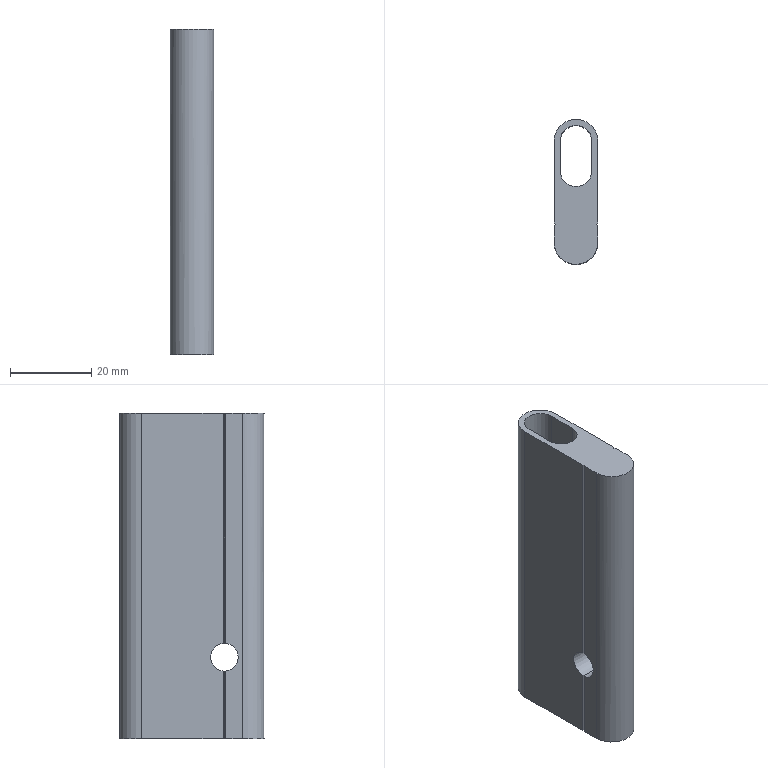Part | STEP file | 46A-01005CC13 | 1 solid | 22 faces | box 10.8 x 35.7 x 80 mm | volume 20059 mm3 | plane 16 | cylinder 6 | commonest cylinder face diameters 6.8 x2 7.8 x2 10.8 x2
STEP:
#1=CARTESIAN_POINT('',(-5.1,-8.,23.4));
#2=VERTEX_POINT('',#1);
#3=CARTESIAN_POINT('',(-5.4,-8.3,23.387));
#4=VERTEX_POINT('',#3);
#5=CARTESIAN_POINT('',(-5.1,-8.,23.4));
#6=CARTESIAN_POINT('',(-5.2,-8.1,23.4));
#7=CARTESIAN_POINT('',(-5.3,-8.2,23.396));
#8=CARTESIAN_POINT('',(-5.4,-8.3,23.387));
#9=B_SPLINE_CURVE_WITH_KNOTS('',3,(#5,#6,#7,#8),.UNSPECIFIED.,.F.,.U.,(4,4),(0.,0.6004),.UNSPECIFIED.);
#10=EDGE_CURVE('',#2,#4,#9,.T.);
#11=ORIENTED_EDGE('',*,*,#10,.F.);
#12=CARTESIAN_POINT('',(5.1,-8.,23.4));
#13=VERTEX_POINT('',#12);
#14=CARTESIAN_POINT('',(5.4,-8.,23.4));
#15=DIRECTION('',(1.,0.,0.));
#16=VECTOR('',#15,1.);
#17=LINE('',#14,#16);
#18=EDGE_CURVE('',#2,#13,#17,.T.);
#19=ORIENTED_EDGE('',*,*,#18,.T.);
#20=CARTESIAN_POINT('',(5.4,-8.3,23.387));
#21=VERTEX_POINT('',#20);
#22=CARTESIAN_POINT('',(5.4,-8.3,23.387));
#23=CARTESIAN_POINT('',(5.3,-8.2,23.396));
#24=CARTESIAN_POINT('',(5.2,-8.1,23.4));
#25=CARTESIAN_POINT('',(5.1,-8.,23.4));
#26=B_SPLINE_CURVE_WITH_KNOTS('',3,(#22,#23,#24,#25),.UNSPECIFIED.,.F.,.U.,(4,4),(0.,0.6004),.UNSPECIFIED.);
#27=EDGE_CURVE('',#21,#13,#26,.T.);
#28=ORIENTED_EDGE('',*,*,#27,.F.);
#29=CARTESIAN_POINT('',(5.4,-8.3,16.613));
#30=VERTEX_POINT('',#29);
#31=CARTESIAN_POINT('',(5.4,-8.,20.));
#32=DIRECTION('',(1.,0.,0.));
#33=AXIS2_PLACEMENT_3D('',#31,#32,$);
#34=CIRCLE('',#33,3.4);
#35=EDGE_CURVE('',#21,#30,#34,.T.);
#36=ORIENTED_EDGE('',*,*,#35,.T.);
#37=CARTESIAN_POINT('',(5.1,-8.,16.6));
#38=VERTEX_POINT('',#37);
#39=CARTESIAN_POINT('',(5.1,-8.,16.6));
#40=CARTESIAN_POINT('',(5.2,-8.1,16.6));
#41=CARTESIAN_POINT('',(5.3,-8.2,16.604));
#42=CARTESIAN_POINT('',(5.4,-8.3,16.613));
#43=B_SPLINE_CURVE_WITH_KNOTS('',3,(#39,#40,#41,#42),.UNSPECIFIED.,.F.,.U.,(4,4),(0.,0.6004),.UNSPECIFIED.);
#44=EDGE_CURVE('',#38,#30,#43,.T.);
#45=ORIENTED_EDGE('',*,*,#44,.F.);
#46=CARTESIAN_POINT('',(-5.1,-8.,16.6));
#47=VERTEX_POINT('',#46);
#48=CARTESIAN_POINT('',(5.4,-8.,16.6));
#49=DIRECTION('',(1.,0.,0.));
#50=VECTOR('',#49,1.);
#51=LINE('',#48,#50);
#52=EDGE_CURVE('',#47,#38,#51,.T.);
#53=ORIENTED_EDGE('',*,*,#52,.F.);
#54=CARTESIAN_POINT('',(-5.4,-8.3,16.613));
#55=VERTEX_POINT('',#54);
#56=CARTESIAN_POINT('',(-5.4,-8.3,16.613));
#57=CARTESIAN_POINT('',(-5.3,-8.2,16.604));
#58=CARTESIAN_POINT('',(-5.2,-8.1,16.6));
#59=CARTESIAN_POINT('',(-5.1,-8.,16.6));
#60=B_SPLINE_CURVE_WITH_KNOTS('',3,(#56,#57,#58,#59),.UNSPECIFIED.,.F.,.U.,(4,4),(0.,0.6004),.UNSPECIFIED.);
#61=EDGE_CURVE('',#55,#47,#60,.T.);
#62=ORIENTED_EDGE('',*,*,#61,.F.);
#63=CARTESIAN_POINT('',(-5.4,-8.,20.));
#64=DIRECTION('',(1.,0.,0.));
#65=AXIS2_PLACEMENT_3D('',#63,#64,$);
#66=CIRCLE('',#65,3.4);
#67=EDGE_CURVE('',#4,#55,#66,.T.);
#68=ORIENTED_EDGE('',*,*,#67,.F.);
#69=EDGE_LOOP('',(#11,#19,#28,#36,#45,#53,#62,#68));
#70=FACE_OUTER_BOUND('',#69,.T.);
#71=CARTESIAN_POINT('',(5.4,-8.,20.));
#72=DIRECTION('',(1.,0.,0.));
#73=DIRECTION('',(0.,0.,1.));
#74=AXIS2_PLACEMENT_3D('',#71,#72,#73);
#75=CYLINDRICAL_SURFACE('',#74,3.4);
#76=ADVANCED_FACE('',(#70),#75,.F.);
#77=CARTESIAN_POINT('',(-5.1,-8.,80.));
#78=VERTEX_POINT('',#77);
#79=CARTESIAN_POINT('',(-5.1,-8.,51.7));
#80=DIRECTION('',(0.,0.,1.));
#81=VECTOR('',#80,1.);
#82=LINE('',#79,#81);
#83=EDGE_CURVE('',#2,#78,#82,.T.);
#84=ORIENTED_EDGE('',*,*,#83,.F.);
#85=ORIENTED_EDGE('',*,*,#10,.T.);
#86=CARTESIAN_POINT('',(-5.4,-8.3,80.));
#87=VERTEX_POINT('',#86);
#88=CARTESIAN_POINT('',(-5.4,-8.3,51.693));
#89=DIRECTION('',(0.,0.,1.));
#90=VECTOR('',#89,1.);
#91=LINE('',#88,#90);
#92=EDGE_CURVE('',#4,#87,#91,.T.);
#93=ORIENTED_EDGE('',*,*,#92,.T.);
#94=CARTESIAN_POINT('',(-5.25,-8.15,80.));
#95=DIRECTION('',(0.7071,0.7071,0.));
#96=VECTOR('',#95,1.);
#97=LINE('',#94,#96);
#98=EDGE_CURVE('',#87,#78,#97,.T.);
#99=ORIENTED_EDGE('',*,*,#98,.T.);
#100=EDGE_LOOP('',(#84,#85,#93,#99));
#101=FACE_OUTER_BOUND('',#100,.T.);
#102=CARTESIAN_POINT('',(-5.4,-8.3,-20.));
#103=DIRECTION('',(0.7071,-0.7071,0.));
#104=DIRECTION('',(0.7071,0.7071,0.));
#105=AXIS2_PLACEMENT_3D('',#102,#103,#104);
#106=PLANE('',#105);
#107=ADVANCED_FACE('',(#101),#106,.F.);
#108=ORIENTED_EDGE('',*,*,#18,.F.);
#109=CARTESIAN_POINT('',(-5.4,-7.7,23.387));
#110=VERTEX_POINT('',#109);
#111=CARTESIAN_POINT('',(-5.4,-7.7,23.387));
#112=CARTESIAN_POINT('',(-5.3,-7.8,23.396));
#113=CARTESIAN_POINT('',(-5.2,-7.9,23.4));
#114=CARTESIAN_POINT('',(-5.1,-8.,23.4));
#115=B_SPLINE_CURVE_WITH_KNOTS('',3,(#111,#112,#113,#114),.UNSPECIFIED.,.F.,.U.,(4,4),(0.,0.6004),.UNSPECIFIED.);
#116=EDGE_CURVE('',#110,#2,#115,.T.);
#117=ORIENTED_EDGE('',*,*,#116,.F.);
#118=CARTESIAN_POINT('',(-5.4,-7.7,16.613));
#119=VERTEX_POINT('',#118);
#120=CARTESIAN_POINT('',(-5.4,-8.,20.));
#121=DIRECTION('',(1.,0.,0.));
#122=AXIS2_PLACEMENT_3D('',#120,#121,$);
#123=CIRCLE('',#122,3.4);
#124=EDGE_CURVE('',#119,#110,#123,.T.);
#125=ORIENTED_EDGE('',*,*,#124,.F.);
#126=CARTESIAN_POINT('',(-5.1,-8.,16.6));
#127=CARTESIAN_POINT('',(-5.2,-7.9,16.6));
#128=CARTESIAN_POINT('',(-5.3,-7.8,16.604));
#129=CARTESIAN_POINT('',(-5.4,-7.7,16.613));
#130=B_SPLINE_CURVE_WITH_KNOTS('',3,(#126,#127,#128,#129),.UNSPECIFIED.,.F.,.U.,(4,4),(0.,0.6004),.UNSPECIFIED.);
#131=EDGE_CURVE('',#47,#119,#130,.T.);
#132=ORIENTED_EDGE('',*,*,#131,.F.);
#133=ORIENTED_EDGE('',*,*,#52,.T.);
#134=CARTESIAN_POINT('',(5.4,-7.7,16.613));
#135=VERTEX_POINT('',#134);
#136=CARTESIAN_POINT('',(5.4,-7.7,16.613));
#137=CARTESIAN_POINT('',(5.3,-7.8,16.604));
#138=CARTESIAN_POINT('',(5.2,-7.9,16.6));
#139=CARTESIAN_POINT('',(5.1,-8.,16.6));
#140=B_SPLINE_CURVE_WITH_KNOTS('',3,(#136,#137,#138,#139),.UNSPECIFIED.,.F.,.U.,(4,4),(0.,0.6004),.UNSPECIFIED.);
#141=EDGE_CURVE('',#135,#38,#140,.T.);
#142=ORIENTED_EDGE('',*,*,#141,.F.);
#143=CARTESIAN_POINT('',(5.4,-7.7,23.387));
#144=VERTEX_POINT('',#143);
#145=CARTESIAN_POINT('',(5.4,-8.,20.));
#146=DIRECTION('',(1.,0.,0.));
#147=AXIS2_PLACEMENT_3D('',#145,#146,$);
#148=CIRCLE('',#147,3.4);
#149=EDGE_CURVE('',#135,#144,#148,.T.);
#150=ORIENTED_EDGE('',*,*,#149,.T.);
#151=CARTESIAN_POINT('',(5.1,-8.,23.4));
#152=CARTESIAN_POINT('',(5.2,-7.9,23.4));
#153=CARTESIAN_POINT('',(5.3,-7.8,23.396));
#154=CARTESIAN_POINT('',(5.4,-7.7,23.387));
#155=B_SPLINE_CURVE_WITH_KNOTS('',3,(#151,#152,#153,#154),.UNSPECIFIED.,.F.,.U.,(4,4),(0.,0.6004),.UNSPECIFIED.);
#156=EDGE_CURVE('',#13,#144,#155,.T.);
#157=ORIENTED_EDGE('',*,*,#156,.F.);
#158=EDGE_LOOP('',(#108,#117,#125,#132,#133,#142,#150,#157));
#159=FACE_OUTER_BOUND('',#158,.T.);
#160=CARTESIAN_POINT('',(5.4,-8.,20.));
#161=DIRECTION('',(1.,0.,0.));
#162=DIRECTION('',(0.,0.,-1.));
#163=AXIS2_PLACEMENT_3D('',#160,#161,#162);
#164=CYLINDRICAL_SURFACE('',#163,3.4);
#165=ADVANCED_FACE('',(#159),#164,.F.);
#166=CARTESIAN_POINT('',(5.4,-8.3,80.));
#167=VERTEX_POINT('',#166);
#168=CARTESIAN_POINT('',(5.4,-8.3,51.693));
#169=DIRECTION('',(0.,0.,1.));
#170=VECTOR('',#169,1.);
#171=LINE('',#168,#170);
#172=EDGE_CURVE('',#21,#167,#171,.T.);
#173=ORIENTED_EDGE('',*,*,#172,.F.);
#174=ORIENTED_EDGE('',*,*,#27,.T.);
#175=CARTESIAN_POINT('',(5.1,-8.,80.));
#176=VERTEX_POINT('',#175);
#177=CARTESIAN_POINT('',(5.1,-8.,51.7));
#178=DIRECTION('',(0.,0.,1.));
#179=VECTOR('',#178,1.);
#180=LINE('',#177,#179);
#181=EDGE_CURVE('',#13,#176,#180,.T.);
#182=ORIENTED_EDGE('',*,*,#181,.T.);
#183=CARTESIAN_POINT('',(5.25,-8.15,80.));
#184=DIRECTION('',(0.7071,-0.7071,0.));
#185=VECTOR('',#184,1.);
#186=LINE('',#183,#185);
#187=EDGE_CURVE('',#176,#167,#186,.T.);
#188=ORIENTED_EDGE('',*,*,#187,.T.);
#189=EDGE_LOOP('',(#173,#174,#182,#188));
#190=FACE_OUTER_BOUND('',#189,.T.);
#191=CARTESIAN_POINT('',(5.4,-8.3,-20.));
#192=DIRECTION('',(-0.7071,-0.7071,0.));
#193=DIRECTION('',(0.7071,-0.7071,0.));
#194=AXIS2_PLACEMENT_3D('',#191,#192,#193);
#195=PLANE('',#194);
#196=ADVANCED_FACE('',(#190),#195,.F.);
#197=CARTESIAN_POINT('',(5.4,-8.3,0.));
#198=VERTEX_POINT('',#197);
#199=CARTESIAN_POINT('',(5.4,-8.3,8.307));
#200=DIRECTION('',(0.,0.,1.));
#201=VECTOR('',#200,1.);
#202=LINE('',#199,#201);
#203=EDGE_CURVE('',#198,#30,#202,.T.);
#204=ORIENTED_EDGE('',*,*,#203,.T.);
#205=ORIENTED_EDGE('',*,*,#35,.F.);
#206=ORIENTED_EDGE('',*,*,#172,.T.);
#207=CARTESIAN_POINT('',(5.4,-12.45,80.));
#208=VERTEX_POINT('',#207);
#209=CARTESIAN_POINT('',(5.4,-10.375,80.));
#210=DIRECTION('',(0.,1.,0.));
#211=VECTOR('',#210,1.);
#212=LINE('',#209,#211);
#213=EDGE_CURVE('',#208,#167,#212,.T.);
#214=ORIENTED_EDGE('',*,*,#213,.F.);
#215=CARTESIAN_POINT('',(5.4,-12.45,0.));
#216=VERTEX_POINT('',#215);
#217=CARTESIAN_POINT('',(5.4,-12.45,40.));
#218=DIRECTION('',(0.,0.,-1.));
#219=VECTOR('',#218,1.);
#220=LINE('',#217,#219);
#221=EDGE_CURVE('',#208,#216,#220,.T.);
#222=ORIENTED_EDGE('',*,*,#221,.T.);
#223=CARTESIAN_POINT('',(5.4,-10.375,0.));
#224=DIRECTION('',(0.,1.,0.));
#225=VECTOR('',#224,1.);
#226=LINE('',#223,#225);
#227=EDGE_CURVE('',#216,#198,#226,.T.);
#228=ORIENTED_EDGE('',*,*,#227,.T.);
#229=EDGE_LOOP('',(#204,#205,#206,#214,#222,#228));
#230=FACE_OUTER_BOUND('',#229,.T.);
#231=CARTESIAN_POINT('',(5.4,-12.45,80.));
#232=DIRECTION('',(-1.,0.,0.));
#233=DIRECTION('',(0.,0.,1.));
#234=AXIS2_PLACEMENT_3D('',#231,#232,#233);
#235=PLANE('',#234);
#236=ADVANCED_FACE('',(#230),#235,.F.);
#237=CARTESIAN_POINT('',(5.1,-8.,0.));
#238=VERTEX_POINT('',#237);
#239=CARTESIAN_POINT('',(5.1,-8.,8.3));
#240=DIRECTION('',(0.,0.,1.));
#241=VECTOR('',#240,1.);
#242=LINE('',#239,#241);
#243=EDGE_CURVE('',#238,#38,#242,.T.);
#244=ORIENTED_EDGE('',*,*,#243,.T.);
#245=ORIENTED_EDGE('',*,*,#44,.T.);
#246=ORIENTED_EDGE('',*,*,#203,.F.);
#247=CARTESIAN_POINT('',(5.25,-8.15,0.));
#248=DIRECTION('',(0.7071,-0.7071,0.));
#249=VECTOR('',#248,1.);
#250=LINE('',#247,#249);
#251=EDGE_CURVE('',#238,#198,#250,.T.);
#252=ORIENTED_EDGE('',*,*,#251,.F.);
#253=EDGE_LOOP('',(#244,#245,#246,#252));
#254=FACE_OUTER_BOUND('',#253,.T.);
#255=CARTESIAN_POINT('',(5.4,-8.3,-20.));
#256=DIRECTION('',(-0.7071,-0.7071,0.));
#257=DIRECTION('',(0.7071,-0.7071,0.));
#258=AXIS2_PLACEMENT_3D('',#255,#256,#257);
#259=PLANE('',#258);
#260=ADVANCED_FACE('',(#254),#259,.F.);
#261=CARTESIAN_POINT('',(-5.4,-8.3,0.));
#262=VERTEX_POINT('',#261);
#263=CARTESIAN_POINT('',(-5.4,-8.3,8.307));
#264=DIRECTION('',(0.,0.,1.));
#265=VECTOR('',#264,1.);
#266=LINE('',#263,#265);
#267=EDGE_CURVE('',#262,#55,#266,.T.);
#268=ORIENTED_EDGE('',*,*,#267,.T.);
#269=ORIENTED_EDGE('',*,*,#61,.T.);
#270=CARTESIAN_POINT('',(-5.1,-8.,0.));
#271=VERTEX_POINT('',#270);
#272=CARTESIAN_POINT('',(-5.1,-8.,8.3));
#273=DIRECTION('',(0.,0.,1.));
#274=VECTOR('',#273,1.);
#275=LINE('',#272,#274);
#276=EDGE_CURVE('',#271,#47,#275,.T.);
#277=ORIENTED_EDGE('',*,*,#276,.F.);
#278=CARTESIAN_POINT('',(-5.25,-8.15,0.));
#279=DIRECTION('',(0.7071,0.7071,0.));
#280=VECTOR('',#279,1.);
#281=LINE('',#278,#280);
#282=EDGE_CURVE('',#262,#271,#281,.T.);
#283=ORIENTED_EDGE('',*,*,#282,.F.);
#284=EDGE_LOOP('',(#268,#269,#277,#283));
#285=FACE_OUTER_BOUND('',#284,.T.);
#286=CARTESIAN_POINT('',(-5.4,-8.3,-20.));
#287=DIRECTION('',(0.7071,-0.7071,0.));
#288=DIRECTION('',(0.7071,0.7071,0.));
#289=AXIS2_PLACEMENT_3D('',#286,#287,#288);
#290=PLANE('',#289);
#291=ADVANCED_FACE('',(#285),#290,.F.);
#292=ORIENTED_EDGE('',*,*,#67,.T.);
#293=ORIENTED_EDGE('',*,*,#267,.F.);
#294=CARTESIAN_POINT('',(-5.4,-12.45,0.));
#295=VERTEX_POINT('',#294);
#296=CARTESIAN_POINT('',(-5.4,-10.375,0.));
#297=DIRECTION('',(0.,1.,0.));
#298=VECTOR('',#297,1.);
#299=LINE('',#296,#298);
#300=EDGE_CURVE('',#295,#262,#299,.T.);
#301=ORIENTED_EDGE('',*,*,#300,.F.);
#302=CARTESIAN_POINT('',(-5.4,-12.45,80.));
#303=VERTEX_POINT('',#302);
#304=CARTESIAN_POINT('',(-5.4,-12.45,40.));
#305=DIRECTION('',(0.,0.,-1.));
#306=VECTOR('',#305,1.);
#307=LINE('',#304,#306);
#308=EDGE_CURVE('',#303,#295,#307,.T.);
#309=ORIENTED_EDGE('',*,*,#308,.F.);
#310=CARTESIAN_POINT('',(-5.4,-10.375,80.));
#311=DIRECTION('',(0.,1.,0.));
#312=VECTOR('',#311,1.);
#313=LINE('',#310,#312);
#314=EDGE_CURVE('',#303,#87,#313,.T.);
#315=ORIENTED_EDGE('',*,*,#314,.T.);
#316=ORIENTED_EDGE('',*,*,#92,.F.);
#317=EDGE_LOOP('',(#292,#293,#301,#309,#315,#316));
#318=FACE_OUTER_BOUND('',#317,.T.);
#319=CARTESIAN_POINT('',(-5.4,-12.45,80.));
#320=DIRECTION('',(-1.,0.,0.));
#321=DIRECTION('',(0.,-1.,0.));
#322=AXIS2_PLACEMENT_3D('',#319,#320,#321);
#323=PLANE('',#322);
#324=ADVANCED_FACE('',(#318),#323,.T.);
#325=CARTESIAN_POINT('',(-5.4,-7.7,80.));
#326=VERTEX_POINT('',#325);
#327=CARTESIAN_POINT('',(-5.4,-7.7,51.693));
#328=DIRECTION('',(0.,0.,1.));
#329=VECTOR('',#328,1.);
#330=LINE('',#327,#329);
#331=EDGE_CURVE('',#110,#326,#330,.T.);
#332=ORIENTED_EDGE('',*,*,#331,.F.);
#333=ORIENTED_EDGE('',*,*,#116,.T.);
#334=ORIENTED_EDGE('',*,*,#83,.T.);
#335=CARTESIAN_POINT('',(-5.25,-7.85,80.));
#336=DIRECTION('',(-0.7071,0.7071,0.));
#337=VECTOR('',#336,1.);
#338=LINE('',#335,#337);
#339=EDGE_CURVE('',#78,#326,#338,.T.);
#340=ORIENTED_EDGE('',*,*,#339,.T.);
#341=EDGE_LOOP('',(#332,#333,#334,#340));
#342=FACE_OUTER_BOUND('',#341,.T.);
#343=CARTESIAN_POINT('',(-5.4,-7.7,-20.));
#344=DIRECTION('',(0.7071,0.7071,0.));
#345=DIRECTION('',(-0.7071,0.7071,0.));
#346=AXIS2_PLACEMENT_3D('',#343,#344,#345);
#347=PLANE('',#346);
#348=ADVANCED_FACE('',(#342),#347,.F.);
#349=CARTESIAN_POINT('',(5.4,-7.7,80.));
#350=VERTEX_POINT('',#349);
#351=CARTESIAN_POINT('',(5.25,-7.85,80.));
#352=DIRECTION('',(-0.7071,-0.7071,0.));
#353=VECTOR('',#352,1.);
#354=LINE('',#351,#353);
#355=EDGE_CURVE('',#350,#176,#354,.T.);
#356=ORIENTED_EDGE('',*,*,#355,.F.);
#357=CARTESIAN_POINT('',(5.4,12.45,80.));
#358=VERTEX_POINT('',#357);
#359=CARTESIAN_POINT('',(5.4,2.375,80.));
#360=DIRECTION('',(0.,1.,0.));
#361=VECTOR('',#360,1.);
#362=LINE('',#359,#361);
#363=EDGE_CURVE('',#350,#358,#362,.T.);
#364=ORIENTED_EDGE('',*,*,#363,.T.);
#365=CARTESIAN_POINT('',(-5.4,12.45,80.));
#366=VERTEX_POINT('',#365);
#367=CARTESIAN_POINT('',(0.,12.45,80.));
#368=DIRECTION('',(0.,0.,1.));
#369=AXIS2_PLACEMENT_3D('',#367,#368,$);
#370=CIRCLE('',#369,5.4);
#371=EDGE_CURVE('',#358,#366,#370,.T.);
#372=ORIENTED_EDGE('',*,*,#371,.T.);
#373=CARTESIAN_POINT('',(-5.4,2.375,80.));
#374=DIRECTION('',(0.,1.,0.));
#375=VECTOR('',#374,1.);
#376=LINE('',#373,#375);
#377=EDGE_CURVE('',#326,#366,#376,.T.);
#378=ORIENTED_EDGE('',*,*,#377,.F.);
#379=ORIENTED_EDGE('',*,*,#339,.F.);
#380=ORIENTED_EDGE('',*,*,#98,.F.);
#381=ORIENTED_EDGE('',*,*,#314,.F.);
#382=CARTESIAN_POINT('',(5.4,-12.45,80.));
#383=CARTESIAN_POINT('',(5.4,-13.019,80.));
#384=CARTESIAN_POINT('',(5.325,-13.588,80.));
#385=CARTESIAN_POINT('',(5.175,-14.144,80.));
#386=CARTESIAN_POINT('',(4.732,-15.204,80.));
#387=CARTESIAN_POINT('',(4.03,-16.112,80.));
#388=CARTESIAN_POINT('',(3.62,-16.517,80.));
#389=CARTESIAN_POINT('',(2.705,-17.21,80.));
#390=CARTESIAN_POINT('',(1.641,-17.642,80.));
#391=CARTESIAN_POINT('',(1.083,-17.786,80.));
#392=CARTESIAN_POINT('',(-0.05662,-17.925,80.));
#393=CARTESIAN_POINT('',(-1.193,-17.763,80.));
#394=CARTESIAN_POINT('',(-1.748,-17.607,80.));
#395=CARTESIAN_POINT('',(-2.803,-17.153,80.));
#396=CARTESIAN_POINT('',(-3.704,-16.442,80.));
#397=CARTESIAN_POINT('',(-4.105,-16.028,80.));
#398=CARTESIAN_POINT('',(-4.775,-15.123,80.));
#399=CARTESIAN_POINT('',(-5.192,-14.079,80.));
#400=CARTESIAN_POINT('',(-5.331,-13.544,80.));
#401=CARTESIAN_POINT('',(-5.4,-12.997,80.));
#402=CARTESIAN_POINT('',(-5.4,-12.45,80.));
#403=B_SPLINE_CURVE_WITH_KNOTS('',5,(#382,#383,#384,#385,#386,#387,#388,#389,#390,#391,#392,#393,#394,#395,#396,#397,#398,#399,#400,#401,#402),.UNSPECIFIED.,.F.,.U.,(6,3,3,3,3,3,6),(0.,4.025,8.05,12.075,16.099,20.124,23.991),.UNSPECIFIED.);
#404=EDGE_CURVE('',#208,#303,#403,.T.);
#405=ORIENTED_EDGE('',*,*,#404,.F.);
#406=ORIENTED_EDGE('',*,*,#213,.T.);
#407=ORIENTED_EDGE('',*,*,#187,.F.);
#408=EDGE_LOOP('',(#356,#364,#372,#378,#379,#380,#381,#405,#406,#407));
#409=FACE_OUTER_BOUND('',#408,.T.);
#410=CARTESIAN_POINT('',(-3.9,5.15,80.));
#411=VERTEX_POINT('',#410);
#412=CARTESIAN_POINT('',(3.9,5.15,80.));
#413=VERTEX_POINT('',#412);
#414=CARTESIAN_POINT('',(0.,5.15,80.));
#415=DIRECTION('',(0.,0.,1.));
#416=AXIS2_PLACEMENT_3D('',#414,#415,$);
#417=CIRCLE('',#416,3.9);
#418=EDGE_CURVE('',#411,#413,#417,.T.);
#419=ORIENTED_EDGE('',*,*,#418,.F.);
#420=CARTESIAN_POINT('',(-3.9,12.45,80.));
#421=VERTEX_POINT('',#420);
#422=CARTESIAN_POINT('',(-3.9,8.8,80.));
#423=DIRECTION('',(0.,-1.,0.));
#424=VECTOR('',#423,1.);
#425=LINE('',#422,#424);
#426=EDGE_CURVE('',#421,#411,#425,.T.);
#427=ORIENTED_EDGE('',*,*,#426,.F.);
#428=CARTESIAN_POINT('',(3.9,12.45,80.));
#429=VERTEX_POINT('',#428);
#430=CARTESIAN_POINT('',(0.,12.45,80.));
#431=DIRECTION('',(0.,0.,1.));
#432=AXIS2_PLACEMENT_3D('',#430,#431,$);
#433=CIRCLE('',#432,3.9);
#434=EDGE_CURVE('',#429,#421,#433,.T.);
#435=ORIENTED_EDGE('',*,*,#434,.F.);
#436=CARTESIAN_POINT('',(3.9,8.8,80.));
#437=DIRECTION('',(0.,1.,0.));
#438=VECTOR('',#437,1.);
#439=LINE('',#436,#438);
#440=EDGE_CURVE('',#413,#429,#439,.T.);
#441=ORIENTED_EDGE('',*,*,#440,.F.);
#442=EDGE_LOOP('',(#419,#427,#435,#441));
#443=FACE_BOUND('',#442,.T.);
#444=CARTESIAN_POINT('',(0.,12.45,80.));
#445=DIRECTION('',(0.,0.,1.));
#446=DIRECTION('',(1.,0.,0.));
#447=AXIS2_PLACEMENT_3D('',#444,#445,#446);
#448=PLANE('',#447);
#449=ADVANCED_FACE('',(#409,#443),#448,.T.);
#450=ORIENTED_EDGE('',*,*,#124,.T.);
#451=ORIENTED_EDGE('',*,*,#331,.T.);
#452=ORIENTED_EDGE('',*,*,#377,.T.);
#453=CARTESIAN_POINT('',(-5.4,12.45,0.));
#454=VERTEX_POINT('',#453);
#455=CARTESIAN_POINT('',(-5.4,12.45,40.));
#456=DIRECTION('',(0.,0.,-1.));
#457=VECTOR('',#456,1.);
#458=LINE('',#455,#457);
#459=EDGE_CURVE('',#366,#454,#458,.T.);
#460=ORIENTED_EDGE('',*,*,#459,.T.);
#461=CARTESIAN_POINT('',(-5.4,-7.7,0.));
#462=VERTEX_POINT('',#461);
#463=CARTESIAN_POINT('',(-5.4,2.375,0.));
#464=DIRECTION('',(0.,1.,0.));
#465=VECTOR('',#464,1.);
#466=LINE('',#463,#465);
#467=EDGE_CURVE('',#462,#454,#466,.T.);
#468=ORIENTED_EDGE('',*,*,#467,.F.);
#469=CARTESIAN_POINT('',(-5.4,-7.7,8.307));
#470=DIRECTION('',(0.,0.,1.));
#471=VECTOR('',#470,1.);
#472=LINE('',#469,#471);
#473=EDGE_CURVE('',#462,#119,#472,.T.);
#474=ORIENTED_EDGE('',*,*,#473,.T.);
#475=EDGE_LOOP('',(#450,#451,#452,#460,#468,#474));
#476=FACE_OUTER_BOUND('',#475,.T.);
#477=CARTESIAN_POINT('',(-5.4,-12.45,80.));
#478=DIRECTION('',(-1.,0.,0.));
#479=DIRECTION('',(0.,-1.,0.));
#480=AXIS2_PLACEMENT_3D('',#477,#478,#479);
#481=PLANE('',#480);
#482=ADVANCED_FACE('',(#476),#481,.T.);
#483=ORIENTED_EDGE('',*,*,#276,.T.);
#484=ORIENTED_EDGE('',*,*,#131,.T.);
#485=ORIENTED_EDGE('',*,*,#473,.F.);
#486=CARTESIAN_POINT('',(-5.25,-7.85,0.));
#487=DIRECTION('',(-0.7071,0.7071,0.));
#488=VECTOR('',#487,1.);
#489=LINE('',#486,#488);
#490=EDGE_CURVE('',#271,#462,#489,.T.);
#491=ORIENTED_EDGE('',*,*,#490,.F.);
#492=EDGE_LOOP('',(#483,#484,#485,#491));
#493=FACE_OUTER_BOUND('',#492,.T.);
#494=CARTESIAN_POINT('',(-5.4,-7.7,-20.));
#495=DIRECTION('',(0.7071,0.7071,0.));
#496=DIRECTION('',(-0.7071,0.7071,0.));
#497=AXIS2_PLACEMENT_3D('',#494,#495,#496);
#498=PLANE('',#497);
#499=ADVANCED_FACE('',(#493),#498,.F.);
#500=CARTESIAN_POINT('',(5.4,-7.7,0.));
#501=VERTEX_POINT('',#500);
#502=CARTESIAN_POINT('',(5.4,-7.7,8.307));
#503=DIRECTION('',(0.,0.,1.));
#504=VECTOR('',#503,1.);
#505=LINE('',#502,#504);
#506=EDGE_CURVE('',#501,#135,#505,.T.);
#507=ORIENTED_EDGE('',*,*,#506,.T.);
#508=ORIENTED_EDGE('',*,*,#141,.T.);
#509=ORIENTED_EDGE('',*,*,#243,.F.);
#510=CARTESIAN_POINT('',(5.25,-7.85,0.));
#511=DIRECTION('',(-0.7071,-0.7071,0.));
#512=VECTOR('',#511,1.);
#513=LINE('',#510,#512);
#514=EDGE_CURVE('',#501,#238,#513,.T.);
#515=ORIENTED_EDGE('',*,*,#514,.F.);
#516=EDGE_LOOP('',(#507,#508,#509,#515));
#517=FACE_OUTER_BOUND('',#516,.T.);
#518=CARTESIAN_POINT('',(5.4,-7.7,-20.));
#519=DIRECTION('',(-0.7071,0.7071,0.));
#520=DIRECTION('',(-0.7071,-0.7071,0.));
#521=AXIS2_PLACEMENT_3D('',#518,#519,#520);
#522=PLANE('',#521);
#523=ADVANCED_FACE('',(#517),#522,.F.);
#524=CARTESIAN_POINT('',(5.4,-7.7,51.693));
#525=DIRECTION('',(0.,0.,1.));
#526=VECTOR('',#525,1.);
#527=LINE('',#524,#526);
#528=EDGE_CURVE('',#144,#350,#527,.T.);
#529=ORIENTED_EDGE('',*,*,#528,.F.);
#530=ORIENTED_EDGE('',*,*,#149,.F.);
#531=ORIENTED_EDGE('',*,*,#506,.F.);
#532=CARTESIAN_POINT('',(5.4,12.45,0.));
#533=VERTEX_POINT('',#532);
#534=CARTESIAN_POINT('',(5.4,2.375,0.));
#535=DIRECTION('',(0.,1.,0.));
#536=VECTOR('',#535,1.);
#537=LINE('',#534,#536);
#538=EDGE_CURVE('',#501,#533,#537,.T.);
#539=ORIENTED_EDGE('',*,*,#538,.T.);
#540=CARTESIAN_POINT('',(5.4,12.45,40.));
#541=DIRECTION('',(0.,0.,-1.));
#542=VECTOR('',#541,1.);
#543=LINE('',#540,#542);
#544=EDGE_CURVE('',#358,#533,#543,.T.);
#545=ORIENTED_EDGE('',*,*,#544,.F.);
#546=ORIENTED_EDGE('',*,*,#363,.F.);
#547=EDGE_LOOP('',(#529,#530,#531,#539,#545,#546));
#548=FACE_OUTER_BOUND('',#547,.T.);
#549=CARTESIAN_POINT('',(5.4,-12.45,80.));
#550=DIRECTION('',(-1.,0.,0.));
#551=DIRECTION('',(0.,0.,1.));
#552=AXIS2_PLACEMENT_3D('',#549,#550,#551);
#553=PLANE('',#552);
#554=ADVANCED_FACE('',(#548),#553,.F.);
#555=ORIENTED_EDGE('',*,*,#181,.F.);
#556=ORIENTED_EDGE('',*,*,#156,.T.);
#557=ORIENTED_EDGE('',*,*,#528,.T.);
#558=ORIENTED_EDGE('',*,*,#355,.T.);
#559=EDGE_LOOP('',(#555,#556,#557,#558));
#560=FACE_OUTER_BOUND('',#559,.T.);
#561=CARTESIAN_POINT('',(5.4,-7.7,-20.));
#562=DIRECTION('',(-0.7071,0.7071,0.));
#563=DIRECTION('',(-0.7071,-0.7071,0.));
#564=AXIS2_PLACEMENT_3D('',#561,#562,#563);
#565=PLANE('',#564);
#566=ADVANCED_FACE('',(#560),#565,.F.);
#567=CARTESIAN_POINT('',(0.,-12.45,0.));
#568=DIRECTION('',(0.,0.,-1.));
#569=AXIS2_PLACEMENT_3D('',#567,#568,$);
#570=CIRCLE('',#569,5.4);
#571=EDGE_CURVE('',#216,#295,#570,.T.);
#572=ORIENTED_EDGE('',*,*,#571,.F.);
#573=ORIENTED_EDGE('',*,*,#221,.F.);
#574=ORIENTED_EDGE('',*,*,#404,.T.);
#575=ORIENTED_EDGE('',*,*,#308,.T.);
#576=EDGE_LOOP('',(#572,#573,#574,#575));
#577=FACE_OUTER_BOUND('',#576,.T.);
#578=CARTESIAN_POINT('',(0.,-12.45,80.));
#579=DIRECTION('',(0.,0.,-1.));
#580=DIRECTION('',(1.,0.,0.));
#581=AXIS2_PLACEMENT_3D('',#578,#579,#580);
#582=CYLINDRICAL_SURFACE('',#581,5.4);
#583=ADVANCED_FACE('',(#577),#582,.T.);
#584=ORIENTED_EDGE('',*,*,#538,.F.);
#585=ORIENTED_EDGE('',*,*,#514,.T.);
#586=ORIENTED_EDGE('',*,*,#251,.T.);
#587=ORIENTED_EDGE('',*,*,#227,.F.);
#588=ORIENTED_EDGE('',*,*,#571,.T.);
#589=ORIENTED_EDGE('',*,*,#300,.T.);
#590=ORIENTED_EDGE('',*,*,#282,.T.);
#591=ORIENTED_EDGE('',*,*,#490,.T.);
#592=ORIENTED_EDGE('',*,*,#467,.T.);
#593=CARTESIAN_POINT('',(0.,12.45,0.));
#594=DIRECTION('',(0.,0.,1.));
#595=AXIS2_PLACEMENT_3D('',#593,#594,$);
#596=CIRCLE('',#595,5.4);
#597=EDGE_CURVE('',#533,#454,#596,.T.);
#598=ORIENTED_EDGE('',*,*,#597,.F.);
#599=EDGE_LOOP('',(#584,#585,#586,#587,#588,#589,#590,#591,#592,#598));
#600=FACE_OUTER_BOUND('',#599,.T.);
#601=CARTESIAN_POINT('',(-3.9,12.45,0.));
#602=VERTEX_POINT('',#601);
#603=CARTESIAN_POINT('',(-3.9,5.15,0.));
#604=VERTEX_POINT('',#603);
#605=CARTESIAN_POINT('',(-3.9,8.8,0.));
#606=DIRECTION('',(0.,-1.,0.));
#607=VECTOR('',#606,1.);
#608=LINE('',#605,#607);
#609=EDGE_CURVE('',#602,#604,#608,.T.);
#610=ORIENTED_EDGE('',*,*,#609,.T.);
#611=CARTESIAN_POINT('',(3.9,5.15,0.));
#612=VERTEX_POINT('',#611);
#613=CARTESIAN_POINT('',(0.,5.15,0.));
#614=DIRECTION('',(0.,0.,1.));
#615=AXIS2_PLACEMENT_3D('',#613,#614,$);
#616=CIRCLE('',#615,3.9);
#617=EDGE_CURVE('',#604,#612,#616,.T.);
#618=ORIENTED_EDGE('',*,*,#617,.T.);
#619=CARTESIAN_POINT('',(3.9,12.45,0.));
#620=VERTEX_POINT('',#619);
#621=CARTESIAN_POINT('',(3.9,8.8,0.));
#622=DIRECTION('',(0.,1.,0.));
#623=VECTOR('',#622,1.);
#624=LINE('',#621,#623);
#625=EDGE_CURVE('',#612,#620,#624,.T.);
#626=ORIENTED_EDGE('',*,*,#625,.T.);
#627=CARTESIAN_POINT('',(0.,12.45,0.));
#628=DIRECTION('',(0.,0.,1.));
#629=AXIS2_PLACEMENT_3D('',#627,#628,$);
#630=CIRCLE('',#629,3.9);
#631=EDGE_CURVE('',#620,#602,#630,.T.);
#632=ORIENTED_EDGE('',*,*,#631,.T.);
#633=EDGE_LOOP('',(#610,#618,#626,#632));
#634=FACE_BOUND('',#633,.T.);
#635=CARTESIAN_POINT('',(0.,12.45,0.));
#636=DIRECTION('',(0.,0.,1.));
#637=DIRECTION('',(1.,0.,0.));
#638=AXIS2_PLACEMENT_3D('',#635,#636,#637);
#639=PLANE('',#638);
#640=ADVANCED_FACE('',(#600,#634),#639,.F.);
#641=ORIENTED_EDGE('',*,*,#597,.T.);
#642=ORIENTED_EDGE('',*,*,#459,.F.);
#643=ORIENTED_EDGE('',*,*,#371,.F.);
#644=ORIENTED_EDGE('',*,*,#544,.T.);
#645=EDGE_LOOP('',(#641,#642,#643,#644));
#646=FACE_OUTER_BOUND('',#645,.T.);
#647=CARTESIAN_POINT('',(0.,12.45,80.));
#648=DIRECTION('',(0.,0.,-1.));
#649=DIRECTION('',(-1.,0.,0.));
#650=AXIS2_PLACEMENT_3D('',#647,#648,#649);
#651=CYLINDRICAL_SURFACE('',#650,5.4);
#652=ADVANCED_FACE('',(#646),#651,.T.);
#653=CARTESIAN_POINT('',(-3.9,5.15,-20.));
#654=DIRECTION('',(0.,0.,1.));
#655=VECTOR('',#654,1.);
#656=LINE('',#653,#655);
#657=EDGE_CURVE('',#604,#411,#656,.T.);
#658=ORIENTED_EDGE('',*,*,#657,.T.);
#659=ORIENTED_EDGE('',*,*,#418,.T.);
#660=CARTESIAN_POINT('',(3.9,5.15,-20.));
#661=DIRECTION('',(0.,0.,1.));
#662=VECTOR('',#661,1.);
#663=LINE('',#660,#662);
#664=EDGE_CURVE('',#612,#413,#663,.T.);
#665=ORIENTED_EDGE('',*,*,#664,.F.);
#666=ORIENTED_EDGE('',*,*,#617,.F.);
#667=EDGE_LOOP('',(#658,#659,#665,#666));
#668=FACE_OUTER_BOUND('',#667,.T.);
#669=CARTESIAN_POINT('',(0.,5.15,-20.));
#670=DIRECTION('',(0.,0.,1.));
#671=DIRECTION('',(-1.,0.,0.));
#672=AXIS2_PLACEMENT_3D('',#669,#670,#671);
#673=CYLINDRICAL_SURFACE('',#672,3.9);
#674=ADVANCED_FACE('',(#668),#673,.F.);
#675=CARTESIAN_POINT('',(-3.9,12.45,40.));
#676=DIRECTION('',(0.,0.,1.));
#677=VECTOR('',#676,1.);
#678=LINE('',#675,#677);
#679=EDGE_CURVE('',#602,#421,#678,.T.);
#680=ORIENTED_EDGE('',*,*,#679,.T.);
#681=ORIENTED_EDGE('',*,*,#426,.T.);
#682=ORIENTED_EDGE('',*,*,#657,.F.);
#683=ORIENTED_EDGE('',*,*,#609,.F.);
#684=EDGE_LOOP('',(#680,#681,#682,#683));
#685=FACE_OUTER_BOUND('',#684,.T.);
#686=CARTESIAN_POINT('',(-3.9,12.45,-20.));
#687=DIRECTION('',(-1.,0.,0.));
#688=DIRECTION('',(0.,-1.,0.));
#689=AXIS2_PLACEMENT_3D('',#686,#687,#688);
#690=PLANE('',#689);
#691=ADVANCED_FACE('',(#685),#690,.F.);
#692=CARTESIAN_POINT('',(3.9,12.45,-20.));
#693=DIRECTION('',(0.,0.,1.));
#694=VECTOR('',#693,1.);
#695=LINE('',#692,#694);
#696=EDGE_CURVE('',#620,#429,#695,.T.);
#697=ORIENTED_EDGE('',*,*,#696,.T.);
#698=ORIENTED_EDGE('',*,*,#434,.T.);
#699=ORIENTED_EDGE('',*,*,#679,.F.);
#700=ORIENTED_EDGE('',*,*,#631,.F.);
#701=EDGE_LOOP('',(#697,#698,#699,#700));
#702=FACE_OUTER_BOUND('',#701,.T.);
#703=CARTESIAN_POINT('',(0.,12.45,-20.));
#704=DIRECTION('',(0.,0.,1.));
#705=DIRECTION('',(1.,0.,0.));
#706=AXIS2_PLACEMENT_3D('',#703,#704,#705);
#707=CYLINDRICAL_SURFACE('',#706,3.9);
#708=ADVANCED_FACE('',(#702),#707,.F.);
#709=ORIENTED_EDGE('',*,*,#664,.T.);
#710=ORIENTED_EDGE('',*,*,#440,.T.);
#711=ORIENTED_EDGE('',*,*,#696,.F.);
#712=ORIENTED_EDGE('',*,*,#625,.F.);
#713=EDGE_LOOP('',(#709,#710,#711,#712));
#714=FACE_OUTER_BOUND('',#713,.T.);
#715=CARTESIAN_POINT('',(3.9,5.15,-20.));
#716=DIRECTION('',(1.,0.,0.));
#717=DIRECTION('',(0.,1.,0.));
#718=AXIS2_PLACEMENT_3D('',#715,#716,#717);
#719=PLANE('',#718);
#720=ADVANCED_FACE('',(#714),#719,.F.);
#721=CLOSED_SHELL('',(#76,#107,#165,#196,#236,#260,#291,#324,#348,#449,#482,#499,#523,#554,#566,#583,#640,#652,#674,#691,#708,#720));
#722=MANIFOLD_SOLID_BREP('',#721);
#723=(LENGTH_UNIT()NAMED_UNIT(*)SI_UNIT(.MILLI.,.METRE.));
#724=UNCERTAINTY_MEASURE_WITH_UNIT(LENGTH_MEASURE(0.005),#723,'','');
#725=(NAMED_UNIT(*)PLANE_ANGLE_UNIT()SI_UNIT($,.RADIAN.));
#726=(NAMED_UNIT(*)SI_UNIT($,.STERADIAN.)SOLID_ANGLE_UNIT());
#727=(GEOMETRIC_REPRESENTATION_CONTEXT(3)GLOBAL_UNCERTAINTY_ASSIGNED_CONTEXT((#724))GLOBAL_UNIT_ASSIGNED_CONTEXT((#723,#725,#726))REPRESENTATION_CONTEXT('',''));
#728=ADVANCED_BREP_SHAPE_REPRESENTATION('',(#722),#727);